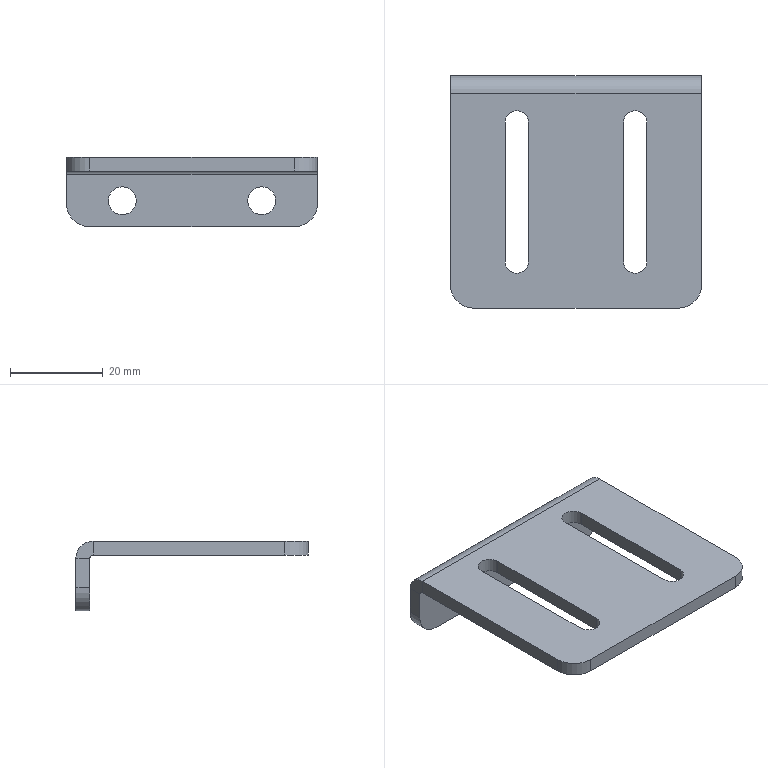Part | SolidWorks | features EdgeFlange 1, Extrusion 1, Fillet 1, FlatPattern 1, ICE 1, SheetMetal 1, SolidToSheetMetal 1 | 1 solid | 30 faces | box 54 x 50 x 15 mm | volume 8636 mm3 | plane 16 | cylinder 14 | commonest cylinder face diameters 5 x4 6 x4 10 x4 1.48 x1 7.48 x1
STEP:
#1=CARTESIAN_POINT('',(42.,-3.,-3.37));
#2=VERTEX_POINT('',#1);
#3=CARTESIAN_POINT('',(42.,-3.,-9.37));
#4=VERTEX_POINT('',#3);
#5=CARTESIAN_POINT('',(42.,-3.,-6.37));
#6=DIRECTION('',(0.,-1.,0.));
#7=DIRECTION('',(0.,0.,-1.));
#8=AXIS2_PLACEMENT_3D('',#5,#6,#7);
#9=CIRCLE('',#8,3.);
#10=EDGE_CURVE('',#2,#4,#9,.T.);
#11=ORIENTED_EDGE('',*,*,#10,.T.);
#12=CARTESIAN_POINT('',(42.,0.,-9.37));
#13=VERTEX_POINT('',#12);
#14=CARTESIAN_POINT('',(42.,-10.,-9.37));
#15=DIRECTION('',(0.,1.,0.));
#16=VECTOR('',#15,1000.);
#17=LINE('',#14,#16);
#18=EDGE_CURVE('',#4,#13,#17,.T.);
#19=ORIENTED_EDGE('',*,*,#18,.T.);
#20=CARTESIAN_POINT('',(42.,0.,-3.37));
#21=VERTEX_POINT('',#20);
#22=CARTESIAN_POINT('',(42.,0.,-6.37));
#23=DIRECTION('',(0.,1.,0.));
#24=DIRECTION('',(0.,0.,1.));
#25=AXIS2_PLACEMENT_3D('',#22,#23,#24);
#26=CIRCLE('',#25,3.);
#27=EDGE_CURVE('',#13,#21,#26,.T.);
#28=ORIENTED_EDGE('',*,*,#27,.T.);
#29=CARTESIAN_POINT('',(42.,-10.,-3.37));
#30=DIRECTION('',(0.,1.,0.));
#31=VECTOR('',#30,1000.);
#32=LINE('',#29,#31);
#33=EDGE_CURVE('',#2,#21,#32,.T.);
#34=ORIENTED_EDGE('',*,*,#33,.F.);
#35=EDGE_LOOP('',(#11,#19,#28,#34));
#36=FACE_OUTER_BOUND('',#35,.T.);
#37=CARTESIAN_POINT('',(42.,-10.,-6.37));
#38=DIRECTION('',(0.,1.,0.));
#39=DIRECTION('',(0.,0.,1.));
#40=AXIS2_PLACEMENT_3D('',#37,#38,#39);
#41=CYLINDRICAL_SURFACE('',#40,3.);
#42=ADVANCED_FACE('',(#36),#41,.F.);
#43=CARTESIAN_POINT('',(12.,-3.,-3.37));
#44=VERTEX_POINT('',#43);
#45=CARTESIAN_POINT('',(12.,-3.,-9.37));
#46=VERTEX_POINT('',#45);
#47=CARTESIAN_POINT('',(12.,-3.,-6.37));
#48=DIRECTION('',(0.,-1.,0.));
#49=DIRECTION('',(0.,0.,-1.));
#50=AXIS2_PLACEMENT_3D('',#47,#48,#49);
#51=CIRCLE('',#50,3.);
#52=EDGE_CURVE('',#44,#46,#51,.T.);
#53=ORIENTED_EDGE('',*,*,#52,.T.);
#54=CARTESIAN_POINT('',(12.,0.,-9.37));
#55=VERTEX_POINT('',#54);
#56=CARTESIAN_POINT('',(12.,-10.,-9.37));
#57=DIRECTION('',(0.,1.,0.));
#58=VECTOR('',#57,1000.);
#59=LINE('',#56,#58);
#60=EDGE_CURVE('',#46,#55,#59,.T.);
#61=ORIENTED_EDGE('',*,*,#60,.T.);
#62=CARTESIAN_POINT('',(12.,0.,-3.37));
#63=VERTEX_POINT('',#62);
#64=CARTESIAN_POINT('',(12.,0.,-6.37));
#65=DIRECTION('',(0.,1.,0.));
#66=DIRECTION('',(0.,0.,1.));
#67=AXIS2_PLACEMENT_3D('',#64,#65,#66);
#68=CIRCLE('',#67,3.);
#69=EDGE_CURVE('',#55,#63,#68,.T.);
#70=ORIENTED_EDGE('',*,*,#69,.T.);
#71=CARTESIAN_POINT('',(12.,-10.,-3.37));
#72=DIRECTION('',(0.,1.,0.));
#73=VECTOR('',#72,1000.);
#74=LINE('',#71,#73);
#75=EDGE_CURVE('',#44,#63,#74,.T.);
#76=ORIENTED_EDGE('',*,*,#75,.F.);
#77=EDGE_LOOP('',(#53,#61,#70,#76));
#78=FACE_OUTER_BOUND('',#77,.T.);
#79=CARTESIAN_POINT('',(12.,-10.,-6.37));
#80=DIRECTION('',(0.,1.,0.));
#81=DIRECTION('',(0.,0.,1.));
#82=AXIS2_PLACEMENT_3D('',#79,#80,#81);
#83=CYLINDRICAL_SURFACE('',#82,3.);
#84=ADVANCED_FACE('',(#78),#83,.F.);
#85=CARTESIAN_POINT('',(54.,-45.,3.));
#86=VERTEX_POINT('',#85);
#87=CARTESIAN_POINT('',(54.,-3.74,3.));
#88=VERTEX_POINT('',#87);
#89=CARTESIAN_POINT('',(54.,0.,3.));
#90=DIRECTION('',(0.,1.,0.));
#91=VECTOR('',#90,1000.);
#92=LINE('',#89,#91);
#93=EDGE_CURVE('',#86,#88,#92,.T.);
#94=ORIENTED_EDGE('',*,*,#93,.F.);
#95=CARTESIAN_POINT('',(54.,-45.,0.));
#96=VERTEX_POINT('',#95);
#97=CARTESIAN_POINT('',(54.,-45.,3.));
#98=DIRECTION('',(0.,0.,-1.));
#99=VECTOR('',#98,1000.);
#100=LINE('',#97,#99);
#101=EDGE_CURVE('',#86,#96,#100,.T.);
#102=ORIENTED_EDGE('',*,*,#101,.T.);
#103=CARTESIAN_POINT('',(54.,-3.74,0.));
#104=VERTEX_POINT('',#103);
#105=CARTESIAN_POINT('',(54.,0.,0.));
#106=DIRECTION('',(0.,1.,0.));
#107=VECTOR('',#106,1000.);
#108=LINE('',#105,#107);
#109=EDGE_CURVE('',#96,#104,#108,.T.);
#110=ORIENTED_EDGE('',*,*,#109,.T.);
#111=CARTESIAN_POINT('',(54.,-3.74,0.));
#112=DIRECTION('',(0.,0.,1.));
#113=VECTOR('',#112,1000.);
#114=LINE('',#111,#113);
#115=EDGE_CURVE('',#104,#88,#114,.T.);
#116=ORIENTED_EDGE('',*,*,#115,.T.);
#117=EDGE_LOOP('',(#94,#102,#110,#116));
#118=FACE_OUTER_BOUND('',#117,.T.);
#119=CARTESIAN_POINT('',(54.,0.,3.));
#120=DIRECTION('',(1.,0.,0.));
#121=DIRECTION('',(0.,1.,0.));
#122=AXIS2_PLACEMENT_3D('',#119,#120,#121);
#123=PLANE('',#122);
#124=ADVANCED_FACE('',(#118),#123,.T.);
#125=CARTESIAN_POINT('',(37.25,-10.,3.));
#126=VERTEX_POINT('',#125);
#127=CARTESIAN_POINT('',(37.25,-40.,3.));
#128=VERTEX_POINT('',#127);
#129=CARTESIAN_POINT('',(37.25,-10.,3.));
#130=DIRECTION('',(0.,-1.,0.));
#131=VECTOR('',#130,1000.);
#132=LINE('',#129,#131);
#133=EDGE_CURVE('',#126,#128,#132,.T.);
#134=ORIENTED_EDGE('',*,*,#133,.F.);
#135=CARTESIAN_POINT('',(42.25,-10.,3.));
#136=VERTEX_POINT('',#135);
#137=CARTESIAN_POINT('',(39.75,-10.,3.));
#138=DIRECTION('',(0.,0.,1.));
#139=DIRECTION('',(1.,0.,0.));
#140=AXIS2_PLACEMENT_3D('',#137,#138,#139);
#141=CIRCLE('',#140,2.5);
#142=EDGE_CURVE('',#136,#126,#141,.T.);
#143=ORIENTED_EDGE('',*,*,#142,.F.);
#144=CARTESIAN_POINT('',(42.25,-40.,3.));
#145=VERTEX_POINT('',#144);
#146=CARTESIAN_POINT('',(42.25,-10.,3.));
#147=DIRECTION('',(0.,1.,0.));
#148=VECTOR('',#147,1000.);
#149=LINE('',#146,#148);
#150=EDGE_CURVE('',#145,#136,#149,.T.);
#151=ORIENTED_EDGE('',*,*,#150,.F.);
#152=CARTESIAN_POINT('',(39.75,-40.,3.));
#153=DIRECTION('',(0.,0.,1.));
#154=DIRECTION('',(1.,0.,0.));
#155=AXIS2_PLACEMENT_3D('',#152,#153,#154);
#156=CIRCLE('',#155,2.5);
#157=EDGE_CURVE('',#128,#145,#156,.T.);
#158=ORIENTED_EDGE('',*,*,#157,.F.);
#159=EDGE_LOOP('',(#134,#143,#151,#158));
#160=FACE_BOUND('',#159,.T.);
#161=CARTESIAN_POINT('',(11.75,-10.,3.));
#162=VERTEX_POINT('',#161);
#163=CARTESIAN_POINT('',(11.75,-40.,3.));
#164=VERTEX_POINT('',#163);
#165=CARTESIAN_POINT('',(11.75,-10.,3.));
#166=DIRECTION('',(0.,-1.,0.));
#167=VECTOR('',#166,1000.);
#168=LINE('',#165,#167);
#169=EDGE_CURVE('',#162,#164,#168,.T.);
#170=ORIENTED_EDGE('',*,*,#169,.F.);
#171=CARTESIAN_POINT('',(16.75,-10.,3.));
#172=VERTEX_POINT('',#171);
#173=CARTESIAN_POINT('',(14.25,-10.,3.));
#174=DIRECTION('',(0.,0.,1.));
#175=DIRECTION('',(-1.,0.,0.));
#176=AXIS2_PLACEMENT_3D('',#173,#174,#175);
#177=CIRCLE('',#176,2.5);
#178=EDGE_CURVE('',#172,#162,#177,.T.);
#179=ORIENTED_EDGE('',*,*,#178,.F.);
#180=CARTESIAN_POINT('',(16.75,-40.,3.));
#181=VERTEX_POINT('',#180);
#182=CARTESIAN_POINT('',(16.75,-10.,3.));
#183=DIRECTION('',(0.,1.,0.));
#184=VECTOR('',#183,1000.);
#185=LINE('',#182,#184);
#186=EDGE_CURVE('',#181,#172,#185,.T.);
#187=ORIENTED_EDGE('',*,*,#186,.F.);
#188=CARTESIAN_POINT('',(14.25,-40.,3.));
#189=DIRECTION('',(0.,0.,1.));
#190=DIRECTION('',(-1.,0.,0.));
#191=AXIS2_PLACEMENT_3D('',#188,#189,#190);
#192=CIRCLE('',#191,2.5);
#193=EDGE_CURVE('',#164,#181,#192,.T.);
#194=ORIENTED_EDGE('',*,*,#193,.F.);
#195=EDGE_LOOP('',(#170,#179,#187,#194));
#196=FACE_BOUND('',#195,.T.);
#197=CARTESIAN_POINT('',(5.,-50.,3.));
#198=VERTEX_POINT('',#197);
#199=CARTESIAN_POINT('',(49.,-50.,3.));
#200=VERTEX_POINT('',#199);
#201=CARTESIAN_POINT('',(0.,-50.,3.));
#202=DIRECTION('',(1.,0.,0.));
#203=VECTOR('',#202,1000.);
#204=LINE('',#201,#203);
#205=EDGE_CURVE('',#198,#200,#204,.T.);
#206=ORIENTED_EDGE('',*,*,#205,.T.);
#207=CARTESIAN_POINT('',(49.,-45.,3.));
#208=DIRECTION('',(0.,0.,1.));
#209=DIRECTION('',(1.,0.,0.));
#210=AXIS2_PLACEMENT_3D('',#207,#208,#209);
#211=CIRCLE('',#210,5.);
#212=EDGE_CURVE('',#200,#86,#211,.T.);
#213=ORIENTED_EDGE('',*,*,#212,.T.);
#214=ORIENTED_EDGE('',*,*,#93,.T.);
#215=CARTESIAN_POINT('',(0.,-3.74,3.));
#216=VERTEX_POINT('',#215);
#217=CARTESIAN_POINT('',(54.,-3.74,3.));
#218=DIRECTION('',(-1.,0.,0.));
#219=VECTOR('',#218,1000.);
#220=LINE('',#217,#219);
#221=EDGE_CURVE('',#88,#216,#220,.T.);
#222=ORIENTED_EDGE('',*,*,#221,.T.);
#223=CARTESIAN_POINT('',(0.,-45.,3.));
#224=VERTEX_POINT('',#223);
#225=CARTESIAN_POINT('',(0.,0.,3.));
#226=DIRECTION('',(0.,-1.,0.));
#227=VECTOR('',#226,1000.);
#228=LINE('',#225,#227);
#229=EDGE_CURVE('',#216,#224,#228,.T.);
#230=ORIENTED_EDGE('',*,*,#229,.T.);
#231=CARTESIAN_POINT('',(5.,-45.,3.));
#232=DIRECTION('',(0.,0.,1.));
#233=DIRECTION('',(1.,0.,0.));
#234=AXIS2_PLACEMENT_3D('',#231,#232,#233);
#235=CIRCLE('',#234,5.);
#236=EDGE_CURVE('',#224,#198,#235,.T.);
#237=ORIENTED_EDGE('',*,*,#236,.T.);
#238=EDGE_LOOP('',(#206,#213,#214,#222,#230,#237));
#239=FACE_OUTER_BOUND('',#238,.T.);
#240=CARTESIAN_POINT('',(0.,0.,3.));
#241=DIRECTION('',(0.,0.,1.));
#242=DIRECTION('',(1.,0.,0.));
#243=AXIS2_PLACEMENT_3D('',#240,#241,#242);
#244=PLANE('',#243);
#245=ADVANCED_FACE('',(#160,#196,#239),#244,.T.);
#246=CARTESIAN_POINT('',(11.75,-10.,0.));
#247=VERTEX_POINT('',#246);
#248=CARTESIAN_POINT('',(11.75,-40.,0.));
#249=VERTEX_POINT('',#248);
#250=CARTESIAN_POINT('',(11.75,0.,0.));
#251=DIRECTION('',(0.,-1.,0.));
#252=VECTOR('',#251,1000.);
#253=LINE('',#250,#252);
#254=EDGE_CURVE('',#247,#249,#253,.T.);
#255=ORIENTED_EDGE('',*,*,#254,.T.);
#256=CARTESIAN_POINT('',(16.75,-40.,0.));
#257=VERTEX_POINT('',#256);
#258=CARTESIAN_POINT('',(14.25,-40.,0.));
#259=DIRECTION('',(0.,0.,1.));
#260=DIRECTION('',(1.,0.,0.));
#261=AXIS2_PLACEMENT_3D('',#258,#259,#260);
#262=CIRCLE('',#261,2.5);
#263=EDGE_CURVE('',#249,#257,#262,.T.);
#264=ORIENTED_EDGE('',*,*,#263,.T.);
#265=CARTESIAN_POINT('',(16.75,-10.,0.));
#266=VERTEX_POINT('',#265);
#267=CARTESIAN_POINT('',(16.75,0.,0.));
#268=DIRECTION('',(0.,1.,0.));
#269=VECTOR('',#268,1000.);
#270=LINE('',#267,#269);
#271=EDGE_CURVE('',#257,#266,#270,.T.);
#272=ORIENTED_EDGE('',*,*,#271,.T.);
#273=CARTESIAN_POINT('',(14.25,-10.,0.));
#274=DIRECTION('',(0.,0.,1.));
#275=DIRECTION('',(1.,0.,0.));
#276=AXIS2_PLACEMENT_3D('',#273,#274,#275);
#277=CIRCLE('',#276,2.5);
#278=EDGE_CURVE('',#266,#247,#277,.T.);
#279=ORIENTED_EDGE('',*,*,#278,.T.);
#280=EDGE_LOOP('',(#255,#264,#272,#279));
#281=FACE_BOUND('',#280,.T.);
#282=CARTESIAN_POINT('',(37.25,-10.,0.));
#283=VERTEX_POINT('',#282);
#284=CARTESIAN_POINT('',(37.25,-40.,0.));
#285=VERTEX_POINT('',#284);
#286=CARTESIAN_POINT('',(37.25,0.,0.));
#287=DIRECTION('',(0.,-1.,0.));
#288=VECTOR('',#287,1000.);
#289=LINE('',#286,#288);
#290=EDGE_CURVE('',#283,#285,#289,.T.);
#291=ORIENTED_EDGE('',*,*,#290,.T.);
#292=CARTESIAN_POINT('',(42.25,-40.,0.));
#293=VERTEX_POINT('',#292);
#294=CARTESIAN_POINT('',(39.75,-40.,0.));
#295=DIRECTION('',(0.,0.,1.));
#296=DIRECTION('',(1.,0.,0.));
#297=AXIS2_PLACEMENT_3D('',#294,#295,#296);
#298=CIRCLE('',#297,2.5);
#299=EDGE_CURVE('',#285,#293,#298,.T.);
#300=ORIENTED_EDGE('',*,*,#299,.T.);
#301=CARTESIAN_POINT('',(42.25,-10.,0.));
#302=VERTEX_POINT('',#301);
#303=CARTESIAN_POINT('',(42.25,0.,0.));
#304=DIRECTION('',(0.,1.,0.));
#305=VECTOR('',#304,1000.);
#306=LINE('',#303,#305);
#307=EDGE_CURVE('',#293,#302,#306,.T.);
#308=ORIENTED_EDGE('',*,*,#307,.T.);
#309=CARTESIAN_POINT('',(39.75,-10.,0.));
#310=DIRECTION('',(0.,0.,1.));
#311=DIRECTION('',(1.,0.,0.));
#312=AXIS2_PLACEMENT_3D('',#309,#310,#311);
#313=CIRCLE('',#312,2.5);
#314=EDGE_CURVE('',#302,#283,#313,.T.);
#315=ORIENTED_EDGE('',*,*,#314,.T.);
#316=EDGE_LOOP('',(#291,#300,#308,#315));
#317=FACE_BOUND('',#316,.T.);
#318=ORIENTED_EDGE('',*,*,#109,.F.);
#319=CARTESIAN_POINT('',(49.,-50.,0.));
#320=VERTEX_POINT('',#319);
#321=CARTESIAN_POINT('',(49.,-45.,0.));
#322=DIRECTION('',(0.,0.,-1.));
#323=DIRECTION('',(1.,0.,0.));
#324=AXIS2_PLACEMENT_3D('',#321,#322,#323);
#325=CIRCLE('',#324,5.);
#326=EDGE_CURVE('',#96,#320,#325,.T.);
#327=ORIENTED_EDGE('',*,*,#326,.T.);
#328=CARTESIAN_POINT('',(5.,-50.,0.));
#329=VERTEX_POINT('',#328);
#330=CARTESIAN_POINT('',(0.,-50.,0.));
#331=DIRECTION('',(1.,0.,0.));
#332=VECTOR('',#331,1000.);
#333=LINE('',#330,#332);
#334=EDGE_CURVE('',#329,#320,#333,.T.);
#335=ORIENTED_EDGE('',*,*,#334,.F.);
#336=CARTESIAN_POINT('',(0.,-45.,0.));
#337=VERTEX_POINT('',#336);
#338=CARTESIAN_POINT('',(5.,-45.,0.));
#339=DIRECTION('',(0.,0.,-1.));
#340=DIRECTION('',(1.,0.,0.));
#341=AXIS2_PLACEMENT_3D('',#338,#339,#340);
#342=CIRCLE('',#341,5.);
#343=EDGE_CURVE('',#329,#337,#342,.T.);
#344=ORIENTED_EDGE('',*,*,#343,.T.);
#345=CARTESIAN_POINT('',(0.,-3.74,0.));
#346=VERTEX_POINT('',#345);
#347=CARTESIAN_POINT('',(0.,0.,0.));
#348=DIRECTION('',(0.,-1.,0.));
#349=VECTOR('',#348,1000.);
#350=LINE('',#347,#349);
#351=EDGE_CURVE('',#346,#337,#350,.T.);
#352=ORIENTED_EDGE('',*,*,#351,.F.);
#353=CARTESIAN_POINT('',(54.,-3.74,0.));
#354=DIRECTION('',(-1.,0.,0.));
#355=VECTOR('',#354,1000.);
#356=LINE('',#353,#355);
#357=EDGE_CURVE('',#104,#346,#356,.T.);
#358=ORIENTED_EDGE('',*,*,#357,.F.);
#359=EDGE_LOOP('',(#318,#327,#335,#344,#352,#358));
#360=FACE_OUTER_BOUND('',#359,.T.);
#361=CARTESIAN_POINT('',(0.,0.,0.));
#362=DIRECTION('',(0.,0.,1.));
#363=DIRECTION('',(1.,0.,0.));
#364=AXIS2_PLACEMENT_3D('',#361,#362,#363);
#365=PLANE('',#364);
#366=ADVANCED_FACE('',(#281,#317,#360),#365,.F.);
#367=CARTESIAN_POINT('',(16.75,-10.,3.));
#368=DIRECTION('',(0.,0.,1.));
#369=VECTOR('',#368,1000.);
#370=LINE('',#367,#369);
#371=EDGE_CURVE('',#266,#172,#370,.T.);
#372=ORIENTED_EDGE('',*,*,#371,.F.);
#373=ORIENTED_EDGE('',*,*,#271,.F.);
#374=CARTESIAN_POINT('',(16.75,-40.,3.));
#375=DIRECTION('',(0.,0.,1.));
#376=VECTOR('',#375,1000.);
#377=LINE('',#374,#376);
#378=EDGE_CURVE('',#257,#181,#377,.T.);
#379=ORIENTED_EDGE('',*,*,#378,.T.);
#380=ORIENTED_EDGE('',*,*,#186,.T.);
#381=EDGE_LOOP('',(#372,#373,#379,#380));
#382=FACE_OUTER_BOUND('',#381,.T.);
#383=CARTESIAN_POINT('',(16.75,-10.,3.));
#384=DIRECTION('',(1.,0.,0.));
#385=DIRECTION('',(0.,1.,0.));
#386=AXIS2_PLACEMENT_3D('',#383,#384,#385);
#387=PLANE('',#386);
#388=ADVANCED_FACE('',(#382),#387,.F.);
#389=ORIENTED_EDGE('',*,*,#378,.F.);
#390=ORIENTED_EDGE('',*,*,#263,.F.);
#391=CARTESIAN_POINT('',(11.75,-40.,3.));
#392=DIRECTION('',(0.,0.,1.));
#393=VECTOR('',#392,1000.);
#394=LINE('',#391,#393);
#395=EDGE_CURVE('',#249,#164,#394,.T.);
#396=ORIENTED_EDGE('',*,*,#395,.T.);
#397=ORIENTED_EDGE('',*,*,#193,.T.);
#398=EDGE_LOOP('',(#389,#390,#396,#397));
#399=FACE_OUTER_BOUND('',#398,.T.);
#400=CARTESIAN_POINT('',(14.25,-40.,3.));
#401=DIRECTION('',(0.,0.,1.));
#402=DIRECTION('',(1.,0.,0.));
#403=AXIS2_PLACEMENT_3D('',#400,#401,#402);
#404=CYLINDRICAL_SURFACE('',#403,2.5);
#405=ADVANCED_FACE('',(#399),#404,.F.);
#406=ORIENTED_EDGE('',*,*,#395,.F.);
#407=ORIENTED_EDGE('',*,*,#254,.F.);
#408=CARTESIAN_POINT('',(11.75,-10.,3.));
#409=DIRECTION('',(0.,0.,1.));
#410=VECTOR('',#409,1000.);
#411=LINE('',#408,#410);
#412=EDGE_CURVE('',#247,#162,#411,.T.);
#413=ORIENTED_EDGE('',*,*,#412,.T.);
#414=ORIENTED_EDGE('',*,*,#169,.T.);
#415=EDGE_LOOP('',(#406,#407,#413,#414));
#416=FACE_OUTER_BOUND('',#415,.T.);
#417=CARTESIAN_POINT('',(11.75,-10.,3.));
#418=DIRECTION('',(-1.,0.,0.));
#419=DIRECTION('',(0.,-1.,0.));
#420=AXIS2_PLACEMENT_3D('',#417,#418,#419);
#421=PLANE('',#420);
#422=ADVANCED_FACE('',(#416),#421,.F.);
#423=CARTESIAN_POINT('',(42.25,-10.,3.));
#424=DIRECTION('',(0.,0.,1.));
#425=VECTOR('',#424,1000.);
#426=LINE('',#423,#425);
#427=EDGE_CURVE('',#302,#136,#426,.T.);
#428=ORIENTED_EDGE('',*,*,#427,.F.);
#429=ORIENTED_EDGE('',*,*,#307,.F.);
#430=CARTESIAN_POINT('',(42.25,-40.,3.));
#431=DIRECTION('',(0.,0.,1.));
#432=VECTOR('',#431,1000.);
#433=LINE('',#430,#432);
#434=EDGE_CURVE('',#293,#145,#433,.T.);
#435=ORIENTED_EDGE('',*,*,#434,.T.);
#436=ORIENTED_EDGE('',*,*,#150,.T.);
#437=EDGE_LOOP('',(#428,#429,#435,#436));
#438=FACE_OUTER_BOUND('',#437,.T.);
#439=CARTESIAN_POINT('',(42.25,-10.,3.));
#440=DIRECTION('',(1.,0.,0.));
#441=DIRECTION('',(0.,1.,0.));
#442=AXIS2_PLACEMENT_3D('',#439,#440,#441);
#443=PLANE('',#442);
#444=ADVANCED_FACE('',(#438),#443,.F.);
#445=ORIENTED_EDGE('',*,*,#434,.F.);
#446=ORIENTED_EDGE('',*,*,#299,.F.);
#447=CARTESIAN_POINT('',(37.25,-40.,3.));
#448=DIRECTION('',(0.,0.,1.));
#449=VECTOR('',#448,1000.);
#450=LINE('',#447,#449);
#451=EDGE_CURVE('',#285,#128,#450,.T.);
#452=ORIENTED_EDGE('',*,*,#451,.T.);
#453=ORIENTED_EDGE('',*,*,#157,.T.);
#454=EDGE_LOOP('',(#445,#446,#452,#453));
#455=FACE_OUTER_BOUND('',#454,.T.);
#456=CARTESIAN_POINT('',(39.75,-40.,3.));
#457=DIRECTION('',(0.,0.,1.));
#458=DIRECTION('',(1.,0.,0.));
#459=AXIS2_PLACEMENT_3D('',#456,#457,#458);
#460=CYLINDRICAL_SURFACE('',#459,2.5);
#461=ADVANCED_FACE('',(#455),#460,.F.);
#462=ORIENTED_EDGE('',*,*,#451,.F.);
#463=ORIENTED_EDGE('',*,*,#290,.F.);
#464=CARTESIAN_POINT('',(37.25,-10.,3.));
#465=DIRECTION('',(0.,0.,1.));
#466=VECTOR('',#465,1000.);
#467=LINE('',#464,#466);
#468=EDGE_CURVE('',#283,#126,#467,.T.);
#469=ORIENTED_EDGE('',*,*,#468,.T.);
#470=ORIENTED_EDGE('',*,*,#133,.T.);
#471=EDGE_LOOP('',(#462,#463,#469,#470));
#472=FACE_OUTER_BOUND('',#471,.T.);
#473=CARTESIAN_POINT('',(37.25,-10.,3.));
#474=DIRECTION('',(-1.,0.,0.));
#475=DIRECTION('',(0.,-1.,0.));
#476=AXIS2_PLACEMENT_3D('',#473,#474,#475);
#477=PLANE('',#476);
#478=ADVANCED_FACE('',(#472),#477,.F.);
#479=ORIENTED_EDGE('',*,*,#351,.T.);
#480=CARTESIAN_POINT('',(0.,-45.,3.));
#481=DIRECTION('',(0.,0.,1.));
#482=VECTOR('',#481,1000.);
#483=LINE('',#480,#482);
#484=EDGE_CURVE('',#337,#224,#483,.T.);
#485=ORIENTED_EDGE('',*,*,#484,.T.);
#486=ORIENTED_EDGE('',*,*,#229,.F.);
#487=CARTESIAN_POINT('',(0.,-3.74,0.));
#488=DIRECTION('',(0.,0.,1.));
#489=VECTOR('',#488,1000.);
#490=LINE('',#487,#489);
#491=EDGE_CURVE('',#346,#216,#490,.T.);
#492=ORIENTED_EDGE('',*,*,#491,.F.);
#493=EDGE_LOOP('',(#479,#485,#486,#492));
#494=FACE_OUTER_BOUND('',#493,.T.);
#495=CARTESIAN_POINT('',(0.,0.,3.));
#496=DIRECTION('',(-1.,0.,0.));
#497=DIRECTION('',(0.,-1.,0.));
#498=AXIS2_PLACEMENT_3D('',#495,#496,#497);
#499=PLANE('',#498);
#500=ADVANCED_FACE('',(#494),#499,.T.);
#501=ORIENTED_EDGE('',*,*,#334,.T.);
#502=CARTESIAN_POINT('',(49.,-50.,3.));
#503=DIRECTION('',(0.,0.,1.));
#504=VECTOR('',#503,1000.);
#505=LINE('',#502,#504);
#506=EDGE_CURVE('',#320,#200,#505,.T.);
#507=ORIENTED_EDGE('',*,*,#506,.T.);
#508=ORIENTED_EDGE('',*,*,#205,.F.);
#509=CARTESIAN_POINT('',(5.,-50.,3.));
#510=DIRECTION('',(0.,0.,-1.));
#511=VECTOR('',#510,1000.);
#512=LINE('',#509,#511);
#513=EDGE_CURVE('',#198,#329,#512,.T.);
#514=ORIENTED_EDGE('',*,*,#513,.T.);
#515=EDGE_LOOP('',(#501,#507,#508,#514));
#516=FACE_OUTER_BOUND('',#515,.T.);
#517=CARTESIAN_POINT('',(0.,-50.,3.));
#518=DIRECTION('',(0.,-1.,0.));
#519=DIRECTION('',(1.,0.,0.));
#520=AXIS2_PLACEMENT_3D('',#517,#518,#519);
#521=PLANE('',#520);
#522=ADVANCED_FACE('',(#516),#521,.T.);
#523=ORIENTED_EDGE('',*,*,#314,.F.);
#524=ORIENTED_EDGE('',*,*,#427,.T.);
#525=ORIENTED_EDGE('',*,*,#142,.T.);
#526=ORIENTED_EDGE('',*,*,#468,.F.);
#527=EDGE_LOOP('',(#523,#524,#525,#526));
#528=FACE_OUTER_BOUND('',#527,.T.);
#529=CARTESIAN_POINT('',(39.75,-10.,3.));
#530=DIRECTION('',(0.,0.,1.));
#531=DIRECTION('',(1.,0.,0.));
#532=AXIS2_PLACEMENT_3D('',#529,#530,#531);
#533=CYLINDRICAL_SURFACE('',#532,2.5);
#534=ADVANCED_FACE('',(#528),#533,.F.);
#535=ORIENTED_EDGE('',*,*,#278,.F.);
#536=ORIENTED_EDGE('',*,*,#371,.T.);
#537=ORIENTED_EDGE('',*,*,#178,.T.);
#538=ORIENTED_EDGE('',*,*,#412,.F.);
#539=EDGE_LOOP('',(#535,#536,#537,#538));
#540=FACE_OUTER_BOUND('',#539,.T.);
#541=CARTESIAN_POINT('',(14.25,-10.,3.));
#542=DIRECTION('',(0.,0.,1.));
#543=DIRECTION('',(1.,0.,0.));
#544=AXIS2_PLACEMENT_3D('',#541,#542,#543);
#545=CYLINDRICAL_SURFACE('',#544,2.5);
#546=ADVANCED_FACE('',(#540),#545,.F.);
#547=CARTESIAN_POINT('',(0.,-3.,-0.74));
#548=VERTEX_POINT('',#547);
#549=CARTESIAN_POINT('',(0.,0.,-0.74));
#550=VERTEX_POINT('',#549);
#551=CARTESIAN_POINT('',(0.,0.,-0.74));
#552=DIRECTION('',(0.,1.,0.));
#553=VECTOR('',#552,1000.);
#554=LINE('',#551,#553);
#555=EDGE_CURVE('',#548,#550,#554,.T.);
#556=ORIENTED_EDGE('',*,*,#555,.F.);
#557=CARTESIAN_POINT('',(0.,-3.74,-0.74));
#558=DIRECTION('',(-1.,0.,0.));
#559=DIRECTION('',(0.,0.,-1.));
#560=AXIS2_PLACEMENT_3D('',#557,#558,#559);
#561=CIRCLE('',#560,0.74);
#562=EDGE_CURVE('',#346,#548,#561,.T.);
#563=ORIENTED_EDGE('',*,*,#562,.F.);
#564=ORIENTED_EDGE('',*,*,#491,.T.);
#565=CARTESIAN_POINT('',(0.,-3.74,-0.74));
#566=DIRECTION('',(-1.,0.,0.));
#567=DIRECTION('',(0.,0.,-1.));
#568=AXIS2_PLACEMENT_3D('',#565,#566,#567);
#569=CIRCLE('',#568,3.74);
#570=EDGE_CURVE('',#216,#550,#569,.T.);
#571=ORIENTED_EDGE('',*,*,#570,.T.);
#572=EDGE_LOOP('',(#556,#563,#564,#571));
#573=FACE_OUTER_BOUND('',#572,.T.);
#574=CARTESIAN_POINT('',(0.,-3.74,-0.74));
#575=DIRECTION('',(-1.,0.,0.));
#576=DIRECTION('',(0.,0.,1.));
#577=AXIS2_PLACEMENT_3D('',#574,#575,#576);
#578=PLANE('',#577);
#579=ADVANCED_FACE('',(#573),#578,.T.);
#580=CARTESIAN_POINT('',(54.,-3.,-0.74));
#581=VERTEX_POINT('',#580);
#582=CARTESIAN_POINT('',(54.,-3.74,-0.74));
#583=DIRECTION('',(1.,0.,0.));
#584=DIRECTION('',(0.,0.,-1.));
#585=AXIS2_PLACEMENT_3D('',#582,#583,#584);
#586=CIRCLE('',#585,0.74);
#587=EDGE_CURVE('',#581,#104,#586,.T.);
#588=ORIENTED_EDGE('',*,*,#587,.F.);
#589=CARTESIAN_POINT('',(54.,0.,-0.74));
#590=VERTEX_POINT('',#589);
#591=CARTESIAN_POINT('',(54.,-3.,-0.74));
#592=DIRECTION('',(0.,1.,0.));
#593=VECTOR('',#592,1000.);
#594=LINE('',#591,#593);
#595=EDGE_CURVE('',#581,#590,#594,.T.);
#596=ORIENTED_EDGE('',*,*,#595,.T.);
#597=CARTESIAN_POINT('',(54.,-3.74,-0.74));
#598=DIRECTION('',(1.,0.,0.));
#599=DIRECTION('',(0.,0.,-1.));
#600=AXIS2_PLACEMENT_3D('',#597,#598,#599);
#601=CIRCLE('',#600,3.74);
#602=EDGE_CURVE('',#590,#88,#601,.T.);
#603=ORIENTED_EDGE('',*,*,#602,.T.);
#604=ORIENTED_EDGE('',*,*,#115,.F.);
#605=EDGE_LOOP('',(#588,#596,#603,#604));
#606=FACE_OUTER_BOUND('',#605,.T.);
#607=CARTESIAN_POINT('',(54.,-3.74,-0.74));
#608=DIRECTION('',(-1.,0.,0.));
#609=DIRECTION('',(0.,0.,1.));
#610=AXIS2_PLACEMENT_3D('',#607,#608,#609);
#611=PLANE('',#610);
#612=ADVANCED_FACE('',(#606),#611,.F.);
#613=ORIENTED_EDGE('',*,*,#221,.F.);
#614=ORIENTED_EDGE('',*,*,#602,.F.);
#615=CARTESIAN_POINT('',(0.,0.,-0.74));
#616=DIRECTION('',(-1.,0.,0.));
#617=VECTOR('',#616,1000.);
#618=LINE('',#615,#617);
#619=EDGE_CURVE('',#590,#550,#618,.T.);
#620=ORIENTED_EDGE('',*,*,#619,.T.);
#621=ORIENTED_EDGE('',*,*,#570,.F.);
#622=EDGE_LOOP('',(#613,#614,#620,#621));
#623=FACE_OUTER_BOUND('',#622,.T.);
#624=CARTESIAN_POINT('',(54.,-3.74,-0.74));
#625=DIRECTION('',(1.,0.,0.));
#626=DIRECTION('',(0.,1.,0.));
#627=AXIS2_PLACEMENT_3D('',#624,#625,#626);
#628=CYLINDRICAL_SURFACE('',#627,3.74);
#629=ADVANCED_FACE('',(#623),#628,.T.);
#630=ORIENTED_EDGE('',*,*,#357,.T.);
#631=ORIENTED_EDGE('',*,*,#562,.T.);
#632=CARTESIAN_POINT('',(0.,-3.,-0.74));
#633=DIRECTION('',(1.,0.,0.));
#634=VECTOR('',#633,1000.);
#635=LINE('',#632,#634);
#636=EDGE_CURVE('',#548,#581,#635,.T.);
#637=ORIENTED_EDGE('',*,*,#636,.T.);
#638=ORIENTED_EDGE('',*,*,#587,.T.);
#639=EDGE_LOOP('',(#630,#631,#637,#638));
#640=FACE_OUTER_BOUND('',#639,.T.);
#641=CARTESIAN_POINT('',(54.,-3.74,-0.74));
#642=DIRECTION('',(1.,0.,0.));
#643=DIRECTION('',(0.,1.,0.));
#644=AXIS2_PLACEMENT_3D('',#641,#642,#643);
#645=CYLINDRICAL_SURFACE('',#644,0.74);
#646=ADVANCED_FACE('',(#640),#645,.F.);
#647=CARTESIAN_POINT('',(54.,-3.,-7.));
#648=VERTEX_POINT('',#647);
#649=CARTESIAN_POINT('',(54.,-3.,-12.));
#650=DIRECTION('',(0.,0.,-1.));
#651=VECTOR('',#650,1000.);
#652=LINE('',#649,#651);
#653=EDGE_CURVE('',#581,#648,#652,.T.);
#654=ORIENTED_EDGE('',*,*,#653,.T.);
#655=CARTESIAN_POINT('',(54.,0.,-7.));
#656=VERTEX_POINT('',#655);
#657=CARTESIAN_POINT('',(54.,0.,-7.));
#658=DIRECTION('',(0.,1.,0.));
#659=VECTOR('',#658,1000.);
#660=LINE('',#657,#659);
#661=EDGE_CURVE('',#648,#656,#660,.T.);
#662=ORIENTED_EDGE('',*,*,#661,.T.);
#663=CARTESIAN_POINT('',(54.,0.,0.));
#664=DIRECTION('',(0.,0.,-1.));
#665=VECTOR('',#664,1000.);
#666=LINE('',#663,#665);
#667=EDGE_CURVE('',#590,#656,#666,.T.);
#668=ORIENTED_EDGE('',*,*,#667,.F.);
#669=ORIENTED_EDGE('',*,*,#595,.F.);
#670=EDGE_LOOP('',(#654,#662,#668,#669));
#671=FACE_OUTER_BOUND('',#670,.T.);
#672=CARTESIAN_POINT('',(54.,0.,-12.));
#673=DIRECTION('',(-1.,0.,0.));
#674=DIRECTION('',(0.,0.,1.));
#675=AXIS2_PLACEMENT_3D('',#672,#673,#674);
#676=PLANE('',#675);
#677=ADVANCED_FACE('',(#671),#676,.F.);
#678=CARTESIAN_POINT('',(0.,0.,-7.));
#679=VERTEX_POINT('',#678);
#680=CARTESIAN_POINT('',(0.,0.,0.));
#681=DIRECTION('',(0.,0.,1.));
#682=VECTOR('',#681,1000.);
#683=LINE('',#680,#682);
#684=EDGE_CURVE('',#679,#550,#683,.T.);
#685=ORIENTED_EDGE('',*,*,#684,.F.);
#686=CARTESIAN_POINT('',(0.,-3.,-7.));
#687=VERTEX_POINT('',#686);
#688=CARTESIAN_POINT('',(0.,0.,-7.));
#689=DIRECTION('',(0.,-1.,0.));
#690=VECTOR('',#689,1000.);
#691=LINE('',#688,#690);
#692=EDGE_CURVE('',#679,#687,#691,.T.);
#693=ORIENTED_EDGE('',*,*,#692,.T.);
#694=CARTESIAN_POINT('',(0.,-3.,0.));
#695=DIRECTION('',(0.,0.,1.));
#696=VECTOR('',#695,1000.);
#697=LINE('',#694,#696);
#698=EDGE_CURVE('',#687,#548,#697,.T.);
#699=ORIENTED_EDGE('',*,*,#698,.T.);
#700=ORIENTED_EDGE('',*,*,#555,.T.);
#701=EDGE_LOOP('',(#685,#693,#699,#700));
#702=FACE_OUTER_BOUND('',#701,.T.);
#703=CARTESIAN_POINT('',(0.,0.,0.));
#704=DIRECTION('',(1.,0.,0.));
#705=DIRECTION('',(0.,0.,-1.));
#706=AXIS2_PLACEMENT_3D('',#703,#704,#705);
#707=PLANE('',#706);
#708=ADVANCED_FACE('',(#702),#707,.F.);
#709=CARTESIAN_POINT('',(42.,0.,-6.37));
#710=DIRECTION('',(0.,1.,0.));
#711=DIRECTION('',(0.,0.,1.));
#712=AXIS2_PLACEMENT_3D('',#709,#710,#711);
#713=CIRCLE('',#712,3.);
#714=EDGE_CURVE('',#21,#13,#713,.T.);
#715=ORIENTED_EDGE('',*,*,#714,.F.);
#716=ORIENTED_EDGE('',*,*,#27,.F.);
#717=EDGE_LOOP('',(#715,#716));
#718=FACE_BOUND('',#717,.T.);
#719=CARTESIAN_POINT('',(12.,0.,-6.37));
#720=DIRECTION('',(0.,1.,0.));
#721=DIRECTION('',(0.,0.,1.));
#722=AXIS2_PLACEMENT_3D('',#719,#720,#721);
#723=CIRCLE('',#722,3.);
#724=EDGE_CURVE('',#63,#55,#723,.T.);
#725=ORIENTED_EDGE('',*,*,#724,.F.);
#726=ORIENTED_EDGE('',*,*,#69,.F.);
#727=EDGE_LOOP('',(#725,#726));
#728=FACE_BOUND('',#727,.T.);
#729=ORIENTED_EDGE('',*,*,#667,.T.);
#730=CARTESIAN_POINT('',(49.,0.,-12.));
#731=VERTEX_POINT('',#730);
#732=CARTESIAN_POINT('',(49.,0.,-7.));
#733=DIRECTION('',(0.,1.,0.));
#734=DIRECTION('',(0.,0.,-1.));
#735=AXIS2_PLACEMENT_3D('',#732,#733,#734);
#736=CIRCLE('',#735,5.);
#737=EDGE_CURVE('',#656,#731,#736,.T.);
#738=ORIENTED_EDGE('',*,*,#737,.T.);
#739=CARTESIAN_POINT('',(5.,0.,-12.));
#740=VERTEX_POINT('',#739);
#741=CARTESIAN_POINT('',(0.,0.,-12.));
#742=DIRECTION('',(-1.,0.,0.));
#743=VECTOR('',#742,1000.);
#744=LINE('',#741,#743);
#745=EDGE_CURVE('',#731,#740,#744,.T.);
#746=ORIENTED_EDGE('',*,*,#745,.T.);
#747=CARTESIAN_POINT('',(5.,0.,-7.));
#748=DIRECTION('',(0.,1.,0.));
#749=DIRECTION('',(0.,0.,-1.));
#750=AXIS2_PLACEMENT_3D('',#747,#748,#749);
#751=CIRCLE('',#750,5.);
#752=EDGE_CURVE('',#740,#679,#751,.T.);
#753=ORIENTED_EDGE('',*,*,#752,.T.);
#754=ORIENTED_EDGE('',*,*,#684,.T.);
#755=ORIENTED_EDGE('',*,*,#619,.F.);
#756=EDGE_LOOP('',(#729,#738,#746,#753,#754,#755));
#757=FACE_OUTER_BOUND('',#756,.T.);
#758=CARTESIAN_POINT('',(0.,0.,0.));
#759=DIRECTION('',(0.,-1.,0.));
#760=DIRECTION('',(0.,0.,-1.));
#761=AXIS2_PLACEMENT_3D('',#758,#759,#760);
#762=PLANE('',#761);
#763=ADVANCED_FACE('',(#718,#728,#757),#762,.F.);
#764=ORIENTED_EDGE('',*,*,#10,.F.);
#765=CARTESIAN_POINT('',(42.,-3.,-6.37));
#766=DIRECTION('',(0.,-1.,0.));
#767=DIRECTION('',(0.,0.,-1.));
#768=AXIS2_PLACEMENT_3D('',#765,#766,#767);
#769=CIRCLE('',#768,3.);
#770=EDGE_CURVE('',#4,#2,#769,.T.);
#771=ORIENTED_EDGE('',*,*,#770,.F.);
#772=EDGE_LOOP('',(#764,#771));
#773=FACE_BOUND('',#772,.T.);
#774=ORIENTED_EDGE('',*,*,#52,.F.);
#775=CARTESIAN_POINT('',(12.,-3.,-6.37));
#776=DIRECTION('',(0.,-1.,0.));
#777=DIRECTION('',(0.,0.,-1.));
#778=AXIS2_PLACEMENT_3D('',#775,#776,#777);
#779=CIRCLE('',#778,3.);
#780=EDGE_CURVE('',#46,#44,#779,.T.);
#781=ORIENTED_EDGE('',*,*,#780,.F.);
#782=EDGE_LOOP('',(#774,#781));
#783=FACE_BOUND('',#782,.T.);
#784=CARTESIAN_POINT('',(49.,-3.,-12.));
#785=VERTEX_POINT('',#784);
#786=CARTESIAN_POINT('',(5.,-3.,-12.));
#787=VERTEX_POINT('',#786);
#788=CARTESIAN_POINT('',(0.,-3.,-12.));
#789=DIRECTION('',(-1.,0.,0.));
#790=VECTOR('',#789,1000.);
#791=LINE('',#788,#790);
#792=EDGE_CURVE('',#785,#787,#791,.T.);
#793=ORIENTED_EDGE('',*,*,#792,.F.);
#794=CARTESIAN_POINT('',(49.,-3.,-7.));
#795=DIRECTION('',(0.,-1.,0.));
#796=DIRECTION('',(0.,0.,-1.));
#797=AXIS2_PLACEMENT_3D('',#794,#795,#796);
#798=CIRCLE('',#797,5.);
#799=EDGE_CURVE('',#785,#648,#798,.T.);
#800=ORIENTED_EDGE('',*,*,#799,.T.);
#801=ORIENTED_EDGE('',*,*,#653,.F.);
#802=ORIENTED_EDGE('',*,*,#636,.F.);
#803=ORIENTED_EDGE('',*,*,#698,.F.);
#804=CARTESIAN_POINT('',(5.,-3.,-7.));
#805=DIRECTION('',(0.,-1.,0.));
#806=DIRECTION('',(0.,0.,-1.));
#807=AXIS2_PLACEMENT_3D('',#804,#805,#806);
#808=CIRCLE('',#807,5.);
#809=EDGE_CURVE('',#687,#787,#808,.T.);
#810=ORIENTED_EDGE('',*,*,#809,.T.);
#811=EDGE_LOOP('',(#793,#800,#801,#802,#803,#810));
#812=FACE_OUTER_BOUND('',#811,.T.);
#813=CARTESIAN_POINT('',(0.,-3.,0.));
#814=DIRECTION('',(0.,-1.,0.));
#815=DIRECTION('',(0.,0.,-1.));
#816=AXIS2_PLACEMENT_3D('',#813,#814,#815);
#817=PLANE('',#816);
#818=ADVANCED_FACE('',(#773,#783,#812),#817,.T.);
#819=ORIENTED_EDGE('',*,*,#745,.F.);
#820=CARTESIAN_POINT('',(49.,0.,-12.));
#821=DIRECTION('',(0.,-1.,0.));
#822=VECTOR('',#821,1000.);
#823=LINE('',#820,#822);
#824=EDGE_CURVE('',#731,#785,#823,.T.);
#825=ORIENTED_EDGE('',*,*,#824,.T.);
#826=ORIENTED_EDGE('',*,*,#792,.T.);
#827=CARTESIAN_POINT('',(5.,0.,-12.));
#828=DIRECTION('',(0.,1.,0.));
#829=VECTOR('',#828,1000.);
#830=LINE('',#827,#829);
#831=EDGE_CURVE('',#787,#740,#830,.T.);
#832=ORIENTED_EDGE('',*,*,#831,.T.);
#833=EDGE_LOOP('',(#819,#825,#826,#832));
#834=FACE_OUTER_BOUND('',#833,.T.);
#835=CARTESIAN_POINT('',(0.,0.,-12.));
#836=DIRECTION('',(0.,0.,1.));
#837=DIRECTION('',(0.,-1.,0.));
#838=AXIS2_PLACEMENT_3D('',#835,#836,#837);
#839=PLANE('',#838);
#840=ADVANCED_FACE('',(#834),#839,.F.);
#841=ORIENTED_EDGE('',*,*,#60,.F.);
#842=ORIENTED_EDGE('',*,*,#780,.T.);
#843=ORIENTED_EDGE('',*,*,#75,.T.);
#844=ORIENTED_EDGE('',*,*,#724,.T.);
#845=EDGE_LOOP('',(#841,#842,#843,#844));
#846=FACE_OUTER_BOUND('',#845,.T.);
#847=CARTESIAN_POINT('',(12.,-10.,-6.37));
#848=DIRECTION('',(0.,1.,0.));
#849=DIRECTION('',(0.,0.,1.));
#850=AXIS2_PLACEMENT_3D('',#847,#848,#849);
#851=CYLINDRICAL_SURFACE('',#850,3.);
#852=ADVANCED_FACE('',(#846),#851,.F.);
#853=ORIENTED_EDGE('',*,*,#18,.F.);
#854=ORIENTED_EDGE('',*,*,#770,.T.);
#855=ORIENTED_EDGE('',*,*,#33,.T.);
#856=ORIENTED_EDGE('',*,*,#714,.T.);
#857=EDGE_LOOP('',(#853,#854,#855,#856));
#858=FACE_OUTER_BOUND('',#857,.T.);
#859=CARTESIAN_POINT('',(42.,-10.,-6.37));
#860=DIRECTION('',(0.,1.,0.));
#861=DIRECTION('',(0.,0.,1.));
#862=AXIS2_PLACEMENT_3D('',#859,#860,#861);
#863=CYLINDRICAL_SURFACE('',#862,3.);
#864=ADVANCED_FACE('',(#858),#863,.F.);
#865=ORIENTED_EDGE('',*,*,#737,.F.);
#866=ORIENTED_EDGE('',*,*,#661,.F.);
#867=ORIENTED_EDGE('',*,*,#799,.F.);
#868=ORIENTED_EDGE('',*,*,#824,.F.);
#869=EDGE_LOOP('',(#865,#866,#867,#868));
#870=FACE_OUTER_BOUND('',#869,.T.);
#871=CARTESIAN_POINT('',(49.,0.,-7.));
#872=DIRECTION('',(0.,-1.,0.));
#873=DIRECTION('',(0.,0.,-1.));
#874=AXIS2_PLACEMENT_3D('',#871,#872,#873);
#875=CYLINDRICAL_SURFACE('',#874,5.);
#876=ADVANCED_FACE('',(#870),#875,.T.);
#877=ORIENTED_EDGE('',*,*,#752,.F.);
#878=ORIENTED_EDGE('',*,*,#831,.F.);
#879=ORIENTED_EDGE('',*,*,#809,.F.);
#880=ORIENTED_EDGE('',*,*,#692,.F.);
#881=EDGE_LOOP('',(#877,#878,#879,#880));
#882=FACE_OUTER_BOUND('',#881,.T.);
#883=CARTESIAN_POINT('',(5.,0.,-7.));
#884=DIRECTION('',(0.,-1.,0.));
#885=DIRECTION('',(0.,0.,-1.));
#886=AXIS2_PLACEMENT_3D('',#883,#884,#885);
#887=CYLINDRICAL_SURFACE('',#886,5.);
#888=ADVANCED_FACE('',(#882),#887,.T.);
#889=ORIENTED_EDGE('',*,*,#326,.F.);
#890=ORIENTED_EDGE('',*,*,#101,.F.);
#891=ORIENTED_EDGE('',*,*,#212,.F.);
#892=ORIENTED_EDGE('',*,*,#506,.F.);
#893=EDGE_LOOP('',(#889,#890,#891,#892));
#894=FACE_OUTER_BOUND('',#893,.T.);
#895=CARTESIAN_POINT('',(49.,-45.,3.));
#896=DIRECTION('',(0.,0.,1.));
#897=DIRECTION('',(1.,0.,0.));
#898=AXIS2_PLACEMENT_3D('',#895,#896,#897);
#899=CYLINDRICAL_SURFACE('',#898,5.);
#900=ADVANCED_FACE('',(#894),#899,.T.);
#901=ORIENTED_EDGE('',*,*,#343,.F.);
#902=ORIENTED_EDGE('',*,*,#513,.F.);
#903=ORIENTED_EDGE('',*,*,#236,.F.);
#904=ORIENTED_EDGE('',*,*,#484,.F.);
#905=EDGE_LOOP('',(#901,#902,#903,#904));
#906=FACE_OUTER_BOUND('',#905,.T.);
#907=CARTESIAN_POINT('',(5.,-45.,3.));
#908=DIRECTION('',(0.,0.,1.));
#909=DIRECTION('',(1.,0.,0.));
#910=AXIS2_PLACEMENT_3D('',#907,#908,#909);
#911=CYLINDRICAL_SURFACE('',#910,5.);
#912=ADVANCED_FACE('',(#906),#911,.T.);
#913=CLOSED_SHELL('',(#42,#84,#124,#245,#366,#388,#405,#422,#444,#461,#478,#500,#522,#534,#546,#579,#612,#629,#646,#677,#708,#763,#818,#840,#852,#864,#876,#888,#900,#912));
#914=MANIFOLD_SOLID_BREP('',#913);
#915=CARTESIAN_POINT('',(0.,0.,0.));
#916=DIRECTION('',(0.,0.,1.));
#917=DIRECTION('',(1.,0.,0.));
#918=AXIS2_PLACEMENT_3D('',#915,#916,#917);
#919=(LENGTH_UNIT()NAMED_UNIT(*)SI_UNIT(.MILLI.,.METRE.));
#920=UNCERTAINTY_MEASURE_WITH_UNIT(LENGTH_MEASURE(0.00001),#919,'','');
#921=(NAMED_UNIT(*)PLANE_ANGLE_UNIT()SI_UNIT($,.RADIAN.));
#922=(NAMED_UNIT(*)SI_UNIT($,.STERADIAN.)SOLID_ANGLE_UNIT());
#923=(GEOMETRIC_REPRESENTATION_CONTEXT(3)GLOBAL_UNCERTAINTY_ASSIGNED_CONTEXT((#920))GLOBAL_UNIT_ASSIGNED_CONTEXT((#919,#921,#922))REPRESENTATION_CONTEXT('',''));
#924=ADVANCED_BREP_SHAPE_REPRESENTATION('',(#914,#918),#923);